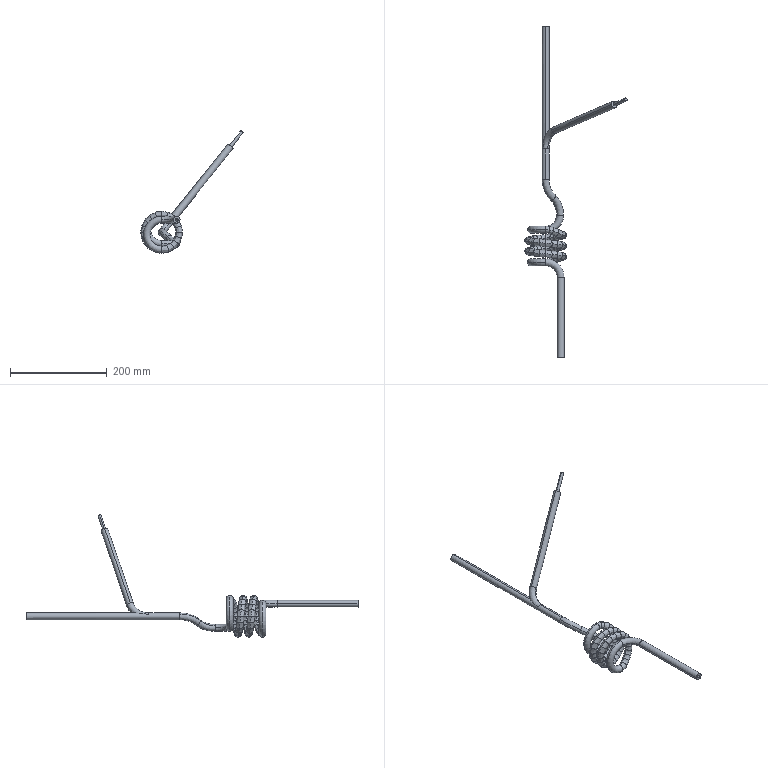Part | NX | features BREP 1 | 1 solid | 248 faces | box 212.038 x 687.689 x 253.179 mm | volume 226070 mm3 | spline 204 | torus 27 | cylinder 12 | plane 5 | commonest cylinder face diameters 6.35 x6 14.3 x6